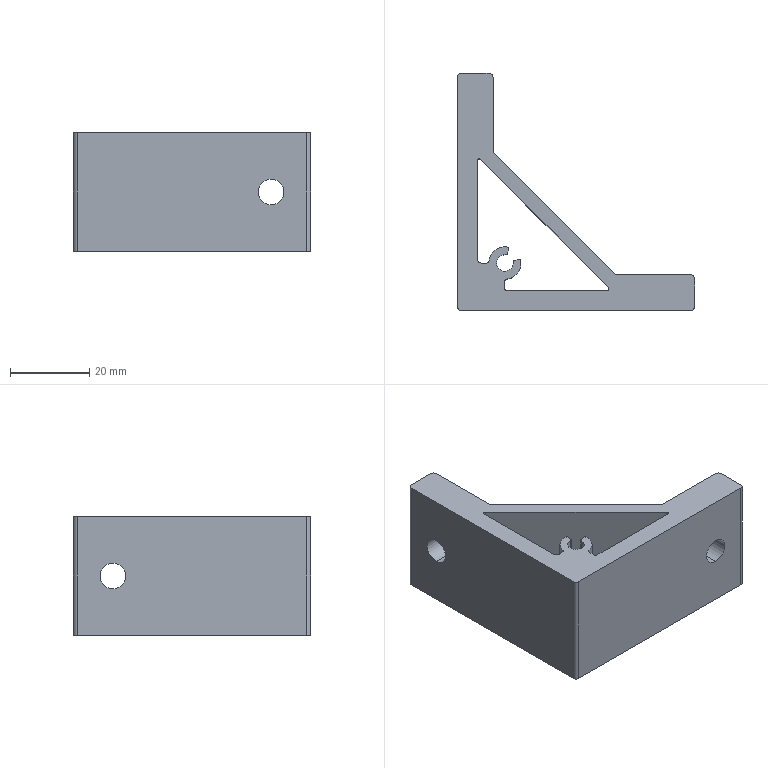Part | SolidWorks | features BaseBody 1 | 1 solid | 41 faces | box 60 x 60 x 30 mm | volume 28435 mm3 | cylinder 25 | plane 16 | commonest cylinder face diameters 1 x10 2 x6 6.5 x4 4.2 x3 8.2 x2
STEP:
#1=CARTESIAN_POINT('',(50.,9.,-11.75));
#2=VERTEX_POINT('',#1);
#3=CARTESIAN_POINT('',(50.,9.,-18.25));
#4=VERTEX_POINT('',#3);
#5=CARTESIAN_POINT('',(50.,9.,-15.));
#6=DIRECTION('',(0.,-1.,0.));
#7=DIRECTION('',(0.,0.,-1.));
#8=AXIS2_PLACEMENT_3D('',#5,#6,#7);
#9=CIRCLE('',#8,3.25);
#10=EDGE_CURVE('',#2,#4,#9,.T.);
#11=ORIENTED_EDGE('',*,*,#10,.F.);
#12=CARTESIAN_POINT('',(50.,0.,-11.75));
#13=VERTEX_POINT('',#12);
#14=CARTESIAN_POINT('',(50.,0.,-11.75));
#15=DIRECTION('',(0.,-1.,0.));
#16=VECTOR('',#15,1000.);
#17=LINE('',#14,#16);
#18=EDGE_CURVE('',#2,#13,#17,.T.);
#19=ORIENTED_EDGE('',*,*,#18,.T.);
#20=CARTESIAN_POINT('',(50.,0.,-18.25));
#21=VERTEX_POINT('',#20);
#22=CARTESIAN_POINT('',(50.,0.,-15.));
#23=DIRECTION('',(0.,1.,0.));
#24=DIRECTION('',(0.,0.,-1.));
#25=AXIS2_PLACEMENT_3D('',#22,#23,#24);
#26=CIRCLE('',#25,3.25);
#27=EDGE_CURVE('',#21,#13,#26,.T.);
#28=ORIENTED_EDGE('',*,*,#27,.F.);
#29=CARTESIAN_POINT('',(50.,0.,-18.25));
#30=DIRECTION('',(0.,-1.,0.));
#31=VECTOR('',#30,1000.);
#32=LINE('',#29,#31);
#33=EDGE_CURVE('',#4,#21,#32,.T.);
#34=ORIENTED_EDGE('',*,*,#33,.F.);
#35=EDGE_LOOP('',(#11,#19,#28,#34));
#36=FACE_OUTER_BOUND('',#35,.T.);
#37=CARTESIAN_POINT('',(50.,0.,-15.));
#38=DIRECTION('',(0.,-1.,0.));
#39=DIRECTION('',(0.,0.,-1.));
#40=AXIS2_PLACEMENT_3D('',#37,#38,#39);
#41=CYLINDRICAL_SURFACE('',#40,3.25);
#42=ADVANCED_FACE('',(#36),#41,.F.);
#43=CARTESIAN_POINT('',(14.101,12.,0.));
#44=VERTEX_POINT('',#43);
#45=CARTESIAN_POINT('',(9.901,12.,0.));
#46=VERTEX_POINT('',#45);
#47=CARTESIAN_POINT('',(12.001,12.,0.));
#48=DIRECTION('',(0.,0.,-1.));
#49=DIRECTION('',(-1.,0.,0.));
#50=AXIS2_PLACEMENT_3D('',#47,#48,#49);
#51=CIRCLE('',#50,2.1);
#52=EDGE_CURVE('',#44,#46,#51,.T.);
#53=ORIENTED_EDGE('',*,*,#52,.F.);
#54=CARTESIAN_POINT('',(14.101,12.,-30.));
#55=VERTEX_POINT('',#54);
#56=CARTESIAN_POINT('',(14.101,12.,-30.));
#57=DIRECTION('',(0.,0.,-1.));
#58=VECTOR('',#57,1000.);
#59=LINE('',#56,#58);
#60=EDGE_CURVE('',#44,#55,#59,.T.);
#61=ORIENTED_EDGE('',*,*,#60,.T.);
#62=CARTESIAN_POINT('',(9.901,12.,-30.));
#63=VERTEX_POINT('',#62);
#64=CARTESIAN_POINT('',(12.001,12.,-30.));
#65=DIRECTION('',(0.,0.,-1.));
#66=DIRECTION('',(-1.,0.,0.));
#67=AXIS2_PLACEMENT_3D('',#64,#65,#66);
#68=CIRCLE('',#67,2.1);
#69=EDGE_CURVE('',#55,#63,#68,.T.);
#70=ORIENTED_EDGE('',*,*,#69,.T.);
#71=CARTESIAN_POINT('',(9.901,12.,-30.));
#72=DIRECTION('',(0.,0.,-1.));
#73=VECTOR('',#72,1000.);
#74=LINE('',#71,#73);
#75=EDGE_CURVE('',#46,#63,#74,.T.);
#76=ORIENTED_EDGE('',*,*,#75,.F.);
#77=EDGE_LOOP('',(#53,#61,#70,#76));
#78=FACE_OUTER_BOUND('',#77,.T.);
#79=CARTESIAN_POINT('',(12.001,12.,-30.));
#80=DIRECTION('',(0.,0.,-1.));
#81=DIRECTION('',(-1.,0.,0.));
#82=AXIS2_PLACEMENT_3D('',#79,#80,#81);
#83=CYLINDRICAL_SURFACE('',#82,2.1);
#84=ADVANCED_FACE('',(#78),#83,.F.);
#85=CARTESIAN_POINT('',(12.144,14.095,0.));
#86=VERTEX_POINT('',#85);
#87=CARTESIAN_POINT('',(12.001,12.,0.));
#88=DIRECTION('',(0.,0.,-1.));
#89=DIRECTION('',(-1.,0.,0.));
#90=AXIS2_PLACEMENT_3D('',#87,#88,#89);
#91=CIRCLE('',#90,2.1);
#92=EDGE_CURVE('',#46,#86,#91,.T.);
#93=ORIENTED_EDGE('',*,*,#92,.F.);
#94=ORIENTED_EDGE('',*,*,#75,.T.);
#95=CARTESIAN_POINT('',(12.144,14.095,-30.));
#96=VERTEX_POINT('',#95);
#97=CARTESIAN_POINT('',(12.001,12.,-30.));
#98=DIRECTION('',(0.,0.,-1.));
#99=DIRECTION('',(-1.,0.,0.));
#100=AXIS2_PLACEMENT_3D('',#97,#98,#99);
#101=CIRCLE('',#100,2.1);
#102=EDGE_CURVE('',#63,#96,#101,.T.);
#103=ORIENTED_EDGE('',*,*,#102,.T.);
#104=CARTESIAN_POINT('',(12.144,14.095,-30.));
#105=DIRECTION('',(0.,0.,-1.));
#106=VECTOR('',#105,1000.);
#107=LINE('',#104,#106);
#108=EDGE_CURVE('',#86,#96,#107,.T.);
#109=ORIENTED_EDGE('',*,*,#108,.F.);
#110=EDGE_LOOP('',(#93,#94,#103,#109));
#111=FACE_OUTER_BOUND('',#110,.T.);
#112=CARTESIAN_POINT('',(12.001,12.,-30.));
#113=DIRECTION('',(0.,0.,-1.));
#114=DIRECTION('',(-1.,0.,0.));
#115=AXIS2_PLACEMENT_3D('',#112,#113,#114);
#116=CYLINDRICAL_SURFACE('',#115,2.1);
#117=ADVANCED_FACE('',(#111),#116,.F.);
#118=CARTESIAN_POINT('',(9.,50.,-11.75));
#119=VERTEX_POINT('',#118);
#120=CARTESIAN_POINT('',(9.,50.,-18.25));
#121=VERTEX_POINT('',#120);
#122=CARTESIAN_POINT('',(9.,50.,-15.));
#123=DIRECTION('',(1.,0.,0.));
#124=DIRECTION('',(0.,0.,1.));
#125=AXIS2_PLACEMENT_3D('',#122,#123,#124);
#126=CIRCLE('',#125,3.25);
#127=EDGE_CURVE('',#119,#121,#126,.T.);
#128=ORIENTED_EDGE('',*,*,#127,.T.);
#129=CARTESIAN_POINT('',(0.,50.,-18.25));
#130=VERTEX_POINT('',#129);
#131=CARTESIAN_POINT('',(0.,50.,-18.25));
#132=DIRECTION('',(-1.,0.,0.));
#133=VECTOR('',#132,1000.);
#134=LINE('',#131,#133);
#135=EDGE_CURVE('',#121,#130,#134,.T.);
#136=ORIENTED_EDGE('',*,*,#135,.T.);
#137=CARTESIAN_POINT('',(0.,50.,-11.75));
#138=VERTEX_POINT('',#137);
#139=CARTESIAN_POINT('',(0.,50.,-15.));
#140=DIRECTION('',(1.,0.,0.));
#141=DIRECTION('',(0.,0.,1.));
#142=AXIS2_PLACEMENT_3D('',#139,#140,#141);
#143=CIRCLE('',#142,3.25);
#144=EDGE_CURVE('',#138,#130,#143,.T.);
#145=ORIENTED_EDGE('',*,*,#144,.F.);
#146=CARTESIAN_POINT('',(0.,50.,-11.75));
#147=DIRECTION('',(-1.,0.,0.));
#148=VECTOR('',#147,1000.);
#149=LINE('',#146,#148);
#150=EDGE_CURVE('',#119,#138,#149,.T.);
#151=ORIENTED_EDGE('',*,*,#150,.F.);
#152=EDGE_LOOP('',(#128,#136,#145,#151));
#153=FACE_OUTER_BOUND('',#152,.T.);
#154=CARTESIAN_POINT('',(0.,50.,-15.));
#155=DIRECTION('',(-1.,0.,0.));
#156=DIRECTION('',(0.,0.,1.));
#157=AXIS2_PLACEMENT_3D('',#154,#155,#156);
#158=CYLINDRICAL_SURFACE('',#157,3.25);
#159=ADVANCED_FACE('',(#153),#158,.F.);
#160=CARTESIAN_POINT('',(14.096,12.143,0.));
#161=VERTEX_POINT('',#160);
#162=CARTESIAN_POINT('',(14.095,12.177,0.));
#163=VERTEX_POINT('',#162);
#164=CARTESIAN_POINT('',(14.595,12.177,0.));
#165=DIRECTION('',(0.,0.,-1.));
#166=DIRECTION('',(-1.,0.,0.));
#167=AXIS2_PLACEMENT_3D('',#164,#165,#166);
#168=CIRCLE('',#167,0.5);
#169=EDGE_CURVE('',#161,#163,#168,.T.);
#170=ORIENTED_EDGE('',*,*,#169,.T.);
#171=CARTESIAN_POINT('',(14.095,12.177,-30.));
#172=VERTEX_POINT('',#171);
#173=CARTESIAN_POINT('',(14.095,12.177,-30.));
#174=DIRECTION('',(0.,0.,-1.));
#175=VECTOR('',#174,1000.);
#176=LINE('',#173,#175);
#177=EDGE_CURVE('',#163,#172,#176,.T.);
#178=ORIENTED_EDGE('',*,*,#177,.T.);
#179=CARTESIAN_POINT('',(14.096,12.143,-30.));
#180=VERTEX_POINT('',#179);
#181=CARTESIAN_POINT('',(14.595,12.177,-30.));
#182=DIRECTION('',(0.,0.,1.));
#183=DIRECTION('',(-1.,0.,0.));
#184=AXIS2_PLACEMENT_3D('',#181,#182,#183);
#185=CIRCLE('',#184,0.5);
#186=EDGE_CURVE('',#172,#180,#185,.T.);
#187=ORIENTED_EDGE('',*,*,#186,.T.);
#188=CARTESIAN_POINT('',(14.096,12.143,-30.));
#189=DIRECTION('',(0.,0.,1.));
#190=VECTOR('',#189,1000.);
#191=LINE('',#188,#190);
#192=EDGE_CURVE('',#180,#161,#191,.T.);
#193=ORIENTED_EDGE('',*,*,#192,.T.);
#194=EDGE_LOOP('',(#170,#178,#187,#193));
#195=FACE_OUTER_BOUND('',#194,.T.);
#196=CARTESIAN_POINT('',(14.595,12.177,-30.));
#197=DIRECTION('',(0.,0.,-1.));
#198=DIRECTION('',(-1.,0.,0.));
#199=AXIS2_PLACEMENT_3D('',#196,#197,#198);
#200=CYLINDRICAL_SURFACE('',#199,0.5);
#201=ADVANCED_FACE('',(#195),#200,.T.);
#202=CARTESIAN_POINT('',(59.,0.,0.));
#203=VERTEX_POINT('',#202);
#204=CARTESIAN_POINT('',(1.,0.,0.));
#205=VERTEX_POINT('',#204);
#206=CARTESIAN_POINT('',(0.,0.,0.));
#207=DIRECTION('',(-1.,0.,0.));
#208=VECTOR('',#207,1000.);
#209=LINE('',#206,#208);
#210=EDGE_CURVE('',#203,#205,#209,.T.);
#211=ORIENTED_EDGE('',*,*,#210,.T.);
#212=CARTESIAN_POINT('',(1.,0.,-30.));
#213=VERTEX_POINT('',#212);
#214=CARTESIAN_POINT('',(1.,0.,-30.));
#215=DIRECTION('',(0.,0.,-1.));
#216=VECTOR('',#215,1000.);
#217=LINE('',#214,#216);
#218=EDGE_CURVE('',#205,#213,#217,.T.);
#219=ORIENTED_EDGE('',*,*,#218,.T.);
#220=CARTESIAN_POINT('',(59.,0.,-30.));
#221=VERTEX_POINT('',#220);
#222=CARTESIAN_POINT('',(0.,0.,-30.));
#223=DIRECTION('',(1.,0.,0.));
#224=VECTOR('',#223,1000.);
#225=LINE('',#222,#224);
#226=EDGE_CURVE('',#213,#221,#225,.T.);
#227=ORIENTED_EDGE('',*,*,#226,.T.);
#228=CARTESIAN_POINT('',(59.,0.,-30.));
#229=DIRECTION('',(0.,0.,1.));
#230=VECTOR('',#229,1000.);
#231=LINE('',#228,#230);
#232=EDGE_CURVE('',#221,#203,#231,.T.);
#233=ORIENTED_EDGE('',*,*,#232,.T.);
#234=EDGE_LOOP('',(#211,#219,#227,#233));
#235=FACE_OUTER_BOUND('',#234,.T.);
#236=ORIENTED_EDGE('',*,*,#27,.T.);
#237=CARTESIAN_POINT('',(50.,0.,-15.));
#238=DIRECTION('',(0.,1.,0.));
#239=DIRECTION('',(0.,0.,-1.));
#240=AXIS2_PLACEMENT_3D('',#237,#238,#239);
#241=CIRCLE('',#240,3.25);
#242=EDGE_CURVE('',#13,#21,#241,.T.);
#243=ORIENTED_EDGE('',*,*,#242,.T.);
#244=EDGE_LOOP('',(#236,#243));
#245=FACE_BOUND('',#244,.T.);
#246=CARTESIAN_POINT('',(0.,0.,-30.));
#247=DIRECTION('',(0.,-1.,0.));
#248=DIRECTION('',(0.,0.,-1.));
#249=AXIS2_PLACEMENT_3D('',#246,#247,#248);
#250=PLANE('',#249);
#251=ADVANCED_FACE('',(#235,#245),#250,.T.);
#252=CARTESIAN_POINT('',(0.,1.,0.));
#253=VERTEX_POINT('',#252);
#254=CARTESIAN_POINT('',(1.,1.,0.));
#255=DIRECTION('',(0.,0.,-1.));
#256=DIRECTION('',(1.,0.,0.));
#257=AXIS2_PLACEMENT_3D('',#254,#255,#256);
#258=CIRCLE('',#257,1.);
#259=EDGE_CURVE('',#205,#253,#258,.T.);
#260=ORIENTED_EDGE('',*,*,#259,.T.);
#261=CARTESIAN_POINT('',(0.,1.,-30.));
#262=VERTEX_POINT('',#261);
#263=CARTESIAN_POINT('',(0.,1.,-30.));
#264=DIRECTION('',(0.,0.,-1.));
#265=VECTOR('',#264,1000.);
#266=LINE('',#263,#265);
#267=EDGE_CURVE('',#253,#262,#266,.T.);
#268=ORIENTED_EDGE('',*,*,#267,.T.);
#269=CARTESIAN_POINT('',(1.,1.,-30.));
#270=DIRECTION('',(0.,0.,1.));
#271=DIRECTION('',(1.,0.,0.));
#272=AXIS2_PLACEMENT_3D('',#269,#270,#271);
#273=CIRCLE('',#272,1.);
#274=EDGE_CURVE('',#262,#213,#273,.T.);
#275=ORIENTED_EDGE('',*,*,#274,.T.);
#276=ORIENTED_EDGE('',*,*,#218,.F.);
#277=EDGE_LOOP('',(#260,#268,#275,#276));
#278=FACE_OUTER_BOUND('',#277,.T.);
#279=CARTESIAN_POINT('',(1.,1.,-30.));
#280=DIRECTION('',(0.,0.,1.));
#281=DIRECTION('',(1.,0.,0.));
#282=AXIS2_PLACEMENT_3D('',#279,#280,#281);
#283=CYLINDRICAL_SURFACE('',#282,1.);
#284=ADVANCED_FACE('',(#278),#283,.T.);
#285=ORIENTED_EDGE('',*,*,#210,.F.);
#286=CARTESIAN_POINT('',(60.,1.,0.));
#287=VERTEX_POINT('',#286);
#288=CARTESIAN_POINT('',(59.,1.,0.));
#289=DIRECTION('',(0.,0.,1.));
#290=DIRECTION('',(1.,0.,0.));
#291=AXIS2_PLACEMENT_3D('',#288,#289,#290);
#292=CIRCLE('',#291,1.);
#293=EDGE_CURVE('',#203,#287,#292,.T.);
#294=ORIENTED_EDGE('',*,*,#293,.T.);
#295=CARTESIAN_POINT('',(60.,8.,0.));
#296=VERTEX_POINT('',#295);
#297=CARTESIAN_POINT('',(60.,0.,0.));
#298=DIRECTION('',(0.,1.,0.));
#299=VECTOR('',#298,1000.);
#300=LINE('',#297,#299);
#301=EDGE_CURVE('',#287,#296,#300,.T.);
#302=ORIENTED_EDGE('',*,*,#301,.T.);
#303=CARTESIAN_POINT('',(59.,9.,0.));
#304=VERTEX_POINT('',#303);
#305=CARTESIAN_POINT('',(59.,8.,0.));
#306=DIRECTION('',(0.,0.,-1.));
#307=DIRECTION('',(1.,0.,0.));
#308=AXIS2_PLACEMENT_3D('',#305,#306,#307);
#309=CIRCLE('',#308,1.);
#310=EDGE_CURVE('',#304,#296,#309,.T.);
#311=ORIENTED_EDGE('',*,*,#310,.F.);
#312=CARTESIAN_POINT('',(40.,9.,0.));
#313=VERTEX_POINT('',#312);
#314=CARTESIAN_POINT('',(0.,9.,0.));
#315=DIRECTION('',(-1.,0.,0.));
#316=VECTOR('',#315,1000.);
#317=LINE('',#314,#316);
#318=EDGE_CURVE('',#304,#313,#317,.T.);
#319=ORIENTED_EDGE('',*,*,#318,.T.);
#320=CARTESIAN_POINT('',(9.,40.,0.));
#321=VERTEX_POINT('',#320);
#322=CARTESIAN_POINT('',(40.,9.,0.));
#323=DIRECTION('',(-0.7071,0.7071,0.));
#324=VECTOR('',#323,1000.);
#325=LINE('',#322,#324);
#326=EDGE_CURVE('',#313,#321,#325,.T.);
#327=ORIENTED_EDGE('',*,*,#326,.T.);
#328=CARTESIAN_POINT('',(9.,59.,0.));
#329=VERTEX_POINT('',#328);
#330=CARTESIAN_POINT('',(9.,0.,0.));
#331=DIRECTION('',(0.,1.,0.));
#332=VECTOR('',#331,1000.);
#333=LINE('',#330,#332);
#334=EDGE_CURVE('',#321,#329,#333,.T.);
#335=ORIENTED_EDGE('',*,*,#334,.T.);
#336=CARTESIAN_POINT('',(8.,60.,0.));
#337=VERTEX_POINT('',#336);
#338=CARTESIAN_POINT('',(8.,59.,0.));
#339=DIRECTION('',(0.,0.,-1.));
#340=DIRECTION('',(1.,0.,0.));
#341=AXIS2_PLACEMENT_3D('',#338,#339,#340);
#342=CIRCLE('',#341,1.);
#343=EDGE_CURVE('',#337,#329,#342,.T.);
#344=ORIENTED_EDGE('',*,*,#343,.F.);
#345=CARTESIAN_POINT('',(1.,60.,0.));
#346=VERTEX_POINT('',#345);
#347=CARTESIAN_POINT('',(0.,60.,0.));
#348=DIRECTION('',(-1.,0.,0.));
#349=VECTOR('',#348,1000.);
#350=LINE('',#347,#349);
#351=EDGE_CURVE('',#337,#346,#350,.T.);
#352=ORIENTED_EDGE('',*,*,#351,.T.);
#353=CARTESIAN_POINT('',(0.,59.,0.));
#354=VERTEX_POINT('',#353);
#355=CARTESIAN_POINT('',(1.,59.,0.));
#356=DIRECTION('',(0.,0.,-1.));
#357=DIRECTION('',(1.,0.,0.));
#358=AXIS2_PLACEMENT_3D('',#355,#356,#357);
#359=CIRCLE('',#358,1.);
#360=EDGE_CURVE('',#354,#346,#359,.T.);
#361=ORIENTED_EDGE('',*,*,#360,.F.);
#362=CARTESIAN_POINT('',(0.,0.,0.));
#363=DIRECTION('',(0.,-1.,0.));
#364=VECTOR('',#363,1000.);
#365=LINE('',#362,#364);
#366=EDGE_CURVE('',#354,#253,#365,.T.);
#367=ORIENTED_EDGE('',*,*,#366,.T.);
#368=ORIENTED_EDGE('',*,*,#259,.F.);
#369=EDGE_LOOP('',(#285,#294,#302,#311,#319,#327,#335,#344,#352,#361,#367,#368));
#370=FACE_OUTER_BOUND('',#369,.T.);
#371=CARTESIAN_POINT('',(12.446,7.924,0.));
#372=VERTEX_POINT('',#371);
#373=CARTESIAN_POINT('',(16.07,12.5,0.));
#374=VERTEX_POINT('',#373);
#375=CARTESIAN_POINT('',(12.001,12.,0.));
#376=DIRECTION('',(0.,0.,1.));
#377=DIRECTION('',(-1.,0.,0.));
#378=AXIS2_PLACEMENT_3D('',#375,#376,#377);
#379=CIRCLE('',#378,4.1);
#380=EDGE_CURVE('',#372,#374,#379,.T.);
#381=ORIENTED_EDGE('',*,*,#380,.T.);
#382=CARTESIAN_POINT('',(15.445,12.922,0.));
#383=VERTEX_POINT('',#382);
#384=CARTESIAN_POINT('',(15.574,12.439,0.));
#385=DIRECTION('',(0.,0.,-1.));
#386=DIRECTION('',(-1.,0.,0.));
#387=AXIS2_PLACEMENT_3D('',#384,#385,#386);
#388=CIRCLE('',#387,0.5);
#389=EDGE_CURVE('',#383,#374,#388,.T.);
#390=ORIENTED_EDGE('',*,*,#389,.F.);
#391=CARTESIAN_POINT('',(14.466,12.66,0.));
#392=VERTEX_POINT('',#391);
#393=CARTESIAN_POINT('',(15.961,13.06,0.));
#394=DIRECTION('',(-0.966,-0.2585,0.));
#395=VECTOR('',#394,1000.);
#396=LINE('',#393,#395);
#397=EDGE_CURVE('',#383,#392,#396,.T.);
#398=ORIENTED_EDGE('',*,*,#397,.T.);
#399=CARTESIAN_POINT('',(14.595,12.177,0.));
#400=DIRECTION('',(0.,0.,-1.));
#401=DIRECTION('',(-1.,0.,0.));
#402=AXIS2_PLACEMENT_3D('',#399,#400,#401);
#403=CIRCLE('',#402,0.5);
#404=EDGE_CURVE('',#163,#392,#403,.T.);
#405=ORIENTED_EDGE('',*,*,#404,.F.);
#406=ORIENTED_EDGE('',*,*,#169,.F.);
#407=CARTESIAN_POINT('',(12.001,12.,0.));
#408=DIRECTION('',(0.,0.,-1.));
#409=DIRECTION('',(-1.,0.,0.));
#410=AXIS2_PLACEMENT_3D('',#407,#408,#409);
#411=CIRCLE('',#410,2.1);
#412=EDGE_CURVE('',#161,#44,#411,.T.);
#413=ORIENTED_EDGE('',*,*,#412,.T.);
#414=ORIENTED_EDGE('',*,*,#52,.T.);
#415=ORIENTED_EDGE('',*,*,#92,.T.);
#416=CARTESIAN_POINT('',(12.661,14.465,0.));
#417=VERTEX_POINT('',#416);
#418=CARTESIAN_POINT('',(12.178,14.594,0.));
#419=DIRECTION('',(0.,0.,-1.));
#420=DIRECTION('',(-1.,0.,0.));
#421=AXIS2_PLACEMENT_3D('',#418,#419,#420);
#422=CIRCLE('',#421,0.5);
#423=EDGE_CURVE('',#417,#86,#422,.T.);
#424=ORIENTED_EDGE('',*,*,#423,.F.);
#425=CARTESIAN_POINT('',(12.923,15.443,0.));
#426=VERTEX_POINT('',#425);
#427=CARTESIAN_POINT('',(12.002,12.001,0.));
#428=DIRECTION('',(0.2585,0.966,0.));
#429=VECTOR('',#428,1000.);
#430=LINE('',#427,#429);
#431=EDGE_CURVE('',#417,#426,#430,.T.);
#432=ORIENTED_EDGE('',*,*,#431,.T.);
#433=CARTESIAN_POINT('',(12.501,16.069,0.));
#434=VERTEX_POINT('',#433);
#435=CARTESIAN_POINT('',(12.44,15.573,0.));
#436=DIRECTION('',(0.,0.,-1.));
#437=DIRECTION('',(-1.,0.,0.));
#438=AXIS2_PLACEMENT_3D('',#435,#436,#437);
#439=CIRCLE('',#438,0.5);
#440=EDGE_CURVE('',#434,#426,#439,.T.);
#441=ORIENTED_EDGE('',*,*,#440,.F.);
#442=CARTESIAN_POINT('',(7.925,12.445,0.));
#443=VERTEX_POINT('',#442);
#444=CARTESIAN_POINT('',(12.001,12.,0.));
#445=DIRECTION('',(0.,0.,1.));
#446=DIRECTION('',(-1.,0.,0.));
#447=AXIS2_PLACEMENT_3D('',#444,#445,#446);
#448=CIRCLE('',#447,4.1);
#449=EDGE_CURVE('',#434,#443,#448,.T.);
#450=ORIENTED_EDGE('',*,*,#449,.T.);
#451=CARTESIAN_POINT('',(7.428,12.,0.));
#452=VERTEX_POINT('',#451);
#453=CARTESIAN_POINT('',(7.428,12.5,0.));
#454=DIRECTION('',(0.,0.,-1.));
#455=DIRECTION('',(-1.,0.,0.));
#456=AXIS2_PLACEMENT_3D('',#453,#454,#455);
#457=CIRCLE('',#456,0.5);
#458=EDGE_CURVE('',#443,#452,#457,.T.);
#459=ORIENTED_EDGE('',*,*,#458,.T.);
#460=CARTESIAN_POINT('',(6.,12.,0.));
#461=VERTEX_POINT('',#460);
#462=CARTESIAN_POINT('',(7.901,12.,0.));
#463=DIRECTION('',(-1.,0.,0.));
#464=VECTOR('',#463,1000.);
#465=LINE('',#462,#464);
#466=EDGE_CURVE('',#452,#461,#465,.T.);
#467=ORIENTED_EDGE('',*,*,#466,.T.);
#468=CARTESIAN_POINT('',(5.,13.,0.));
#469=VERTEX_POINT('',#468);
#470=CARTESIAN_POINT('',(6.,13.,0.));
#471=DIRECTION('',(0.,0.,-1.));
#472=DIRECTION('',(1.,0.,0.));
#473=AXIS2_PLACEMENT_3D('',#470,#471,#472);
#474=CIRCLE('',#473,1.);
#475=EDGE_CURVE('',#461,#469,#474,.T.);
#476=ORIENTED_EDGE('',*,*,#475,.T.);
#477=CARTESIAN_POINT('',(5.,37.843,0.));
#478=VERTEX_POINT('',#477);
#479=CARTESIAN_POINT('',(5.,0.,0.));
#480=DIRECTION('',(0.,1.,0.));
#481=VECTOR('',#480,1000.);
#482=LINE('',#479,#481);
#483=EDGE_CURVE('',#469,#478,#482,.T.);
#484=ORIENTED_EDGE('',*,*,#483,.T.);
#485=CARTESIAN_POINT('',(5.854,38.196,0.));
#486=VERTEX_POINT('',#485);
#487=CARTESIAN_POINT('',(5.5,37.843,0.));
#488=DIRECTION('',(0.,0.,-1.));
#489=DIRECTION('',(-1.,0.,0.));
#490=AXIS2_PLACEMENT_3D('',#487,#488,#489);
#491=CIRCLE('',#490,0.5);
#492=EDGE_CURVE('',#478,#486,#491,.T.);
#493=ORIENTED_EDGE('',*,*,#492,.T.);
#494=CARTESIAN_POINT('',(38.196,5.854,0.));
#495=VERTEX_POINT('',#494);
#496=CARTESIAN_POINT('',(5.854,38.196,0.));
#497=DIRECTION('',(0.7071,-0.7071,0.));
#498=VECTOR('',#497,1000.);
#499=LINE('',#496,#498);
#500=EDGE_CURVE('',#486,#495,#499,.T.);
#501=ORIENTED_EDGE('',*,*,#500,.T.);
#502=CARTESIAN_POINT('',(37.844,5.,0.));
#503=VERTEX_POINT('',#502);
#504=CARTESIAN_POINT('',(37.843,5.5,0.));
#505=DIRECTION('',(0.,0.,-1.));
#506=DIRECTION('',(-1.,0.,0.));
#507=AXIS2_PLACEMENT_3D('',#504,#505,#506);
#508=CIRCLE('',#507,0.5);
#509=EDGE_CURVE('',#495,#503,#508,.T.);
#510=ORIENTED_EDGE('',*,*,#509,.T.);
#511=CARTESIAN_POINT('',(12.5,5.,0.));
#512=VERTEX_POINT('',#511);
#513=CARTESIAN_POINT('',(0.,5.,0.));
#514=DIRECTION('',(-1.,0.,0.));
#515=VECTOR('',#514,1000.);
#516=LINE('',#513,#515);
#517=EDGE_CURVE('',#503,#512,#516,.T.);
#518=ORIENTED_EDGE('',*,*,#517,.T.);
#519=CARTESIAN_POINT('',(12.,5.5,0.));
#520=VERTEX_POINT('',#519);
#521=CARTESIAN_POINT('',(12.5,5.5,0.));
#522=DIRECTION('',(0.,0.,-1.));
#523=DIRECTION('',(1.,0.,0.));
#524=AXIS2_PLACEMENT_3D('',#521,#522,#523);
#525=CIRCLE('',#524,0.5);
#526=EDGE_CURVE('',#512,#520,#525,.T.);
#527=ORIENTED_EDGE('',*,*,#526,.T.);
#528=CARTESIAN_POINT('',(12.,7.427,0.));
#529=VERTEX_POINT('',#528);
#530=CARTESIAN_POINT('',(12.,0.,0.));
#531=DIRECTION('',(0.,1.,0.));
#532=VECTOR('',#531,1000.);
#533=LINE('',#530,#532);
#534=EDGE_CURVE('',#520,#529,#533,.T.);
#535=ORIENTED_EDGE('',*,*,#534,.T.);
#536=CARTESIAN_POINT('',(12.5,7.427,0.));
#537=DIRECTION('',(0.,0.,-1.));
#538=DIRECTION('',(-1.,0.,0.));
#539=AXIS2_PLACEMENT_3D('',#536,#537,#538);
#540=CIRCLE('',#539,0.5);
#541=EDGE_CURVE('',#529,#372,#540,.T.);
#542=ORIENTED_EDGE('',*,*,#541,.T.);
#543=EDGE_LOOP('',(#381,#390,#398,#405,#406,#413,#414,#415,#424,#432,#441,#450,#459,#467,#476,#484,#493,#501,#510,#518,#527,#535,#542));
#544=FACE_BOUND('',#543,.T.);
#545=CARTESIAN_POINT('',(0.,0.,0.));
#546=DIRECTION('',(0.,0.,1.));
#547=DIRECTION('',(1.,0.,0.));
#548=AXIS2_PLACEMENT_3D('',#545,#546,#547);
#549=PLANE('',#548);
#550=ADVANCED_FACE('',(#370,#544),#549,.T.);
#551=ORIENTED_EDGE('',*,*,#293,.F.);
#552=ORIENTED_EDGE('',*,*,#232,.F.);
#553=CARTESIAN_POINT('',(60.,1.,-30.));
#554=VERTEX_POINT('',#553);
#555=CARTESIAN_POINT('',(59.,1.,-30.));
#556=DIRECTION('',(0.,0.,1.));
#557=DIRECTION('',(1.,0.,0.));
#558=AXIS2_PLACEMENT_3D('',#555,#556,#557);
#559=CIRCLE('',#558,1.);
#560=EDGE_CURVE('',#221,#554,#559,.T.);
#561=ORIENTED_EDGE('',*,*,#560,.T.);
#562=CARTESIAN_POINT('',(60.,1.,-30.));
#563=DIRECTION('',(0.,0.,1.));
#564=VECTOR('',#563,1000.);
#565=LINE('',#562,#564);
#566=EDGE_CURVE('',#554,#287,#565,.T.);
#567=ORIENTED_EDGE('',*,*,#566,.T.);
#568=EDGE_LOOP('',(#551,#552,#561,#567));
#569=FACE_OUTER_BOUND('',#568,.T.);
#570=CARTESIAN_POINT('',(59.,1.,-30.));
#571=DIRECTION('',(0.,0.,1.));
#572=DIRECTION('',(1.,0.,0.));
#573=AXIS2_PLACEMENT_3D('',#570,#571,#572);
#574=CYLINDRICAL_SURFACE('',#573,1.);
#575=ADVANCED_FACE('',(#569),#574,.T.);
#576=CARTESIAN_POINT('',(60.,8.,-30.));
#577=VERTEX_POINT('',#576);
#578=CARTESIAN_POINT('',(59.,9.,-30.));
#579=VERTEX_POINT('',#578);
#580=CARTESIAN_POINT('',(59.,8.,-30.));
#581=DIRECTION('',(0.,0.,1.));
#582=DIRECTION('',(1.,0.,0.));
#583=AXIS2_PLACEMENT_3D('',#580,#581,#582);
#584=CIRCLE('',#583,1.);
#585=EDGE_CURVE('',#577,#579,#584,.T.);
#586=ORIENTED_EDGE('',*,*,#585,.F.);
#587=CARTESIAN_POINT('',(60.,0.,-30.));
#588=DIRECTION('',(0.,1.,0.));
#589=VECTOR('',#588,1000.);
#590=LINE('',#587,#589);
#591=EDGE_CURVE('',#554,#577,#590,.T.);
#592=ORIENTED_EDGE('',*,*,#591,.F.);
#593=ORIENTED_EDGE('',*,*,#560,.F.);
#594=ORIENTED_EDGE('',*,*,#226,.F.);
#595=ORIENTED_EDGE('',*,*,#274,.F.);
#596=CARTESIAN_POINT('',(0.,59.,-30.));
#597=VERTEX_POINT('',#596);
#598=CARTESIAN_POINT('',(0.,0.,-30.));
#599=DIRECTION('',(0.,-1.,0.));
#600=VECTOR('',#599,1000.);
#601=LINE('',#598,#600);
#602=EDGE_CURVE('',#597,#262,#601,.T.);
#603=ORIENTED_EDGE('',*,*,#602,.F.);
#604=CARTESIAN_POINT('',(1.,60.,-30.));
#605=VERTEX_POINT('',#604);
#606=CARTESIAN_POINT('',(1.,59.,-30.));
#607=DIRECTION('',(0.,0.,1.));
#608=DIRECTION('',(1.,0.,0.));
#609=AXIS2_PLACEMENT_3D('',#606,#607,#608);
#610=CIRCLE('',#609,1.);
#611=EDGE_CURVE('',#605,#597,#610,.T.);
#612=ORIENTED_EDGE('',*,*,#611,.F.);
#613=CARTESIAN_POINT('',(8.,60.,-30.));
#614=VERTEX_POINT('',#613);
#615=CARTESIAN_POINT('',(0.,60.,-30.));
#616=DIRECTION('',(-1.,0.,0.));
#617=VECTOR('',#616,1000.);
#618=LINE('',#615,#617);
#619=EDGE_CURVE('',#614,#605,#618,.T.);
#620=ORIENTED_EDGE('',*,*,#619,.F.);
#621=CARTESIAN_POINT('',(9.,59.,-30.));
#622=VERTEX_POINT('',#621);
#623=CARTESIAN_POINT('',(8.,59.,-30.));
#624=DIRECTION('',(0.,0.,1.));
#625=DIRECTION('',(1.,0.,0.));
#626=AXIS2_PLACEMENT_3D('',#623,#624,#625);
#627=CIRCLE('',#626,1.);
#628=EDGE_CURVE('',#622,#614,#627,.T.);
#629=ORIENTED_EDGE('',*,*,#628,.F.);
#630=CARTESIAN_POINT('',(9.,40.,-30.));
#631=VERTEX_POINT('',#630);
#632=CARTESIAN_POINT('',(9.,0.,-30.));
#633=DIRECTION('',(0.,1.,0.));
#634=VECTOR('',#633,1000.);
#635=LINE('',#632,#634);
#636=EDGE_CURVE('',#631,#622,#635,.T.);
#637=ORIENTED_EDGE('',*,*,#636,.F.);
#638=CARTESIAN_POINT('',(40.,9.,-30.));
#639=VERTEX_POINT('',#638);
#640=CARTESIAN_POINT('',(40.,9.,-30.));
#641=DIRECTION('',(-0.7071,0.7071,0.));
#642=VECTOR('',#641,1000.);
#643=LINE('',#640,#642);
#644=EDGE_CURVE('',#639,#631,#643,.T.);
#645=ORIENTED_EDGE('',*,*,#644,.F.);
#646=CARTESIAN_POINT('',(0.,9.,-30.));
#647=DIRECTION('',(-1.,0.,0.));
#648=VECTOR('',#647,1000.);
#649=LINE('',#646,#648);
#650=EDGE_CURVE('',#579,#639,#649,.T.);
#651=ORIENTED_EDGE('',*,*,#650,.F.);
#652=EDGE_LOOP('',(#586,#592,#593,#594,#595,#603,#612,#620,#629,#637,#645,#651));
#653=FACE_OUTER_BOUND('',#652,.T.);
#654=CARTESIAN_POINT('',(14.466,12.66,-30.));
#655=VERTEX_POINT('',#654);
#656=CARTESIAN_POINT('',(14.595,12.177,-30.));
#657=DIRECTION('',(0.,0.,1.));
#658=DIRECTION('',(-1.,0.,0.));
#659=AXIS2_PLACEMENT_3D('',#656,#657,#658);
#660=CIRCLE('',#659,0.5);
#661=EDGE_CURVE('',#655,#172,#660,.T.);
#662=ORIENTED_EDGE('',*,*,#661,.F.);
#663=CARTESIAN_POINT('',(15.445,12.922,-30.));
#664=VERTEX_POINT('',#663);
#665=CARTESIAN_POINT('',(15.961,13.06,-30.));
#666=DIRECTION('',(0.966,0.2585,0.));
#667=VECTOR('',#666,1000.);
#668=LINE('',#665,#667);
#669=EDGE_CURVE('',#655,#664,#668,.T.);
#670=ORIENTED_EDGE('',*,*,#669,.T.);
#671=CARTESIAN_POINT('',(16.07,12.5,-30.));
#672=VERTEX_POINT('',#671);
#673=CARTESIAN_POINT('',(15.574,12.439,-30.));
#674=DIRECTION('',(0.,0.,1.));
#675=DIRECTION('',(-1.,0.,0.));
#676=AXIS2_PLACEMENT_3D('',#673,#674,#675);
#677=CIRCLE('',#676,0.5);
#678=EDGE_CURVE('',#672,#664,#677,.T.);
#679=ORIENTED_EDGE('',*,*,#678,.F.);
#680=CARTESIAN_POINT('',(12.446,7.924,-30.));
#681=VERTEX_POINT('',#680);
#682=CARTESIAN_POINT('',(12.001,12.,-30.));
#683=DIRECTION('',(0.,0.,1.));
#684=DIRECTION('',(-1.,0.,0.));
#685=AXIS2_PLACEMENT_3D('',#682,#683,#684);
#686=CIRCLE('',#685,4.1);
#687=EDGE_CURVE('',#681,#672,#686,.T.);
#688=ORIENTED_EDGE('',*,*,#687,.F.);
#689=CARTESIAN_POINT('',(12.,7.427,-30.));
#690=VERTEX_POINT('',#689);
#691=CARTESIAN_POINT('',(12.5,7.427,-30.));
#692=DIRECTION('',(0.,0.,1.));
#693=DIRECTION('',(-1.,0.,0.));
#694=AXIS2_PLACEMENT_3D('',#691,#692,#693);
#695=CIRCLE('',#694,0.5);
#696=EDGE_CURVE('',#681,#690,#695,.T.);
#697=ORIENTED_EDGE('',*,*,#696,.T.);
#698=CARTESIAN_POINT('',(12.,5.5,-30.));
#699=VERTEX_POINT('',#698);
#700=CARTESIAN_POINT('',(12.,0.,-30.));
#701=DIRECTION('',(0.,1.,0.));
#702=VECTOR('',#701,1000.);
#703=LINE('',#700,#702);
#704=EDGE_CURVE('',#699,#690,#703,.T.);
#705=ORIENTED_EDGE('',*,*,#704,.F.);
#706=CARTESIAN_POINT('',(12.5,5.,-30.));
#707=VERTEX_POINT('',#706);
#708=CARTESIAN_POINT('',(12.5,5.5,-30.));
#709=DIRECTION('',(0.,0.,1.));
#710=DIRECTION('',(1.,0.,0.));
#711=AXIS2_PLACEMENT_3D('',#708,#709,#710);
#712=CIRCLE('',#711,0.5);
#713=EDGE_CURVE('',#699,#707,#712,.T.);
#714=ORIENTED_EDGE('',*,*,#713,.T.);
#715=CARTESIAN_POINT('',(37.844,5.,-30.));
#716=VERTEX_POINT('',#715);
#717=CARTESIAN_POINT('',(0.,5.,-30.));
#718=DIRECTION('',(-1.,0.,0.));
#719=VECTOR('',#718,1000.);
#720=LINE('',#717,#719);
#721=EDGE_CURVE('',#716,#707,#720,.T.);
#722=ORIENTED_EDGE('',*,*,#721,.F.);
#723=CARTESIAN_POINT('',(38.196,5.854,-30.));
#724=VERTEX_POINT('',#723);
#725=CARTESIAN_POINT('',(37.843,5.5,-30.));
#726=DIRECTION('',(0.,0.,1.));
#727=DIRECTION('',(-1.,0.,0.));
#728=AXIS2_PLACEMENT_3D('',#725,#726,#727);
#729=CIRCLE('',#728,0.5);
#730=EDGE_CURVE('',#716,#724,#729,.T.);
#731=ORIENTED_EDGE('',*,*,#730,.T.);
#732=CARTESIAN_POINT('',(5.854,38.196,-30.));
#733=VERTEX_POINT('',#732);
#734=CARTESIAN_POINT('',(5.854,38.196,-30.));
#735=DIRECTION('',(0.7071,-0.7071,0.));
#736=VECTOR('',#735,1000.);
#737=LINE('',#734,#736);
#738=EDGE_CURVE('',#733,#724,#737,.T.);
#739=ORIENTED_EDGE('',*,*,#738,.F.);
#740=CARTESIAN_POINT('',(5.,37.843,-30.));
#741=VERTEX_POINT('',#740);
#742=CARTESIAN_POINT('',(5.5,37.843,-30.));
#743=DIRECTION('',(0.,0.,1.));
#744=DIRECTION('',(-1.,0.,0.));
#745=AXIS2_PLACEMENT_3D('',#742,#743,#744);
#746=CIRCLE('',#745,0.5);
#747=EDGE_CURVE('',#733,#741,#746,.T.);
#748=ORIENTED_EDGE('',*,*,#747,.T.);
#749=CARTESIAN_POINT('',(5.,13.,-30.));
#750=VERTEX_POINT('',#749);
#751=CARTESIAN_POINT('',(5.,0.,-30.));
#752=DIRECTION('',(0.,1.,0.));
#753=VECTOR('',#752,1000.);
#754=LINE('',#751,#753);
#755=EDGE_CURVE('',#750,#741,#754,.T.);
#756=ORIENTED_EDGE('',*,*,#755,.F.);
#757=CARTESIAN_POINT('',(6.,12.,-30.));
#758=VERTEX_POINT('',#757);
#759=CARTESIAN_POINT('',(6.,13.,-30.));
#760=DIRECTION('',(0.,0.,1.));
#761=DIRECTION('',(1.,0.,0.));
#762=AXIS2_PLACEMENT_3D('',#759,#760,#761);
#763=CIRCLE('',#762,1.);
#764=EDGE_CURVE('',#750,#758,#763,.T.);
#765=ORIENTED_EDGE('',*,*,#764,.T.);
#766=CARTESIAN_POINT('',(7.428,12.,-30.));
#767=VERTEX_POINT('',#766);
#768=CARTESIAN_POINT('',(7.901,12.,-30.));
#769=DIRECTION('',(1.,0.,0.));
#770=VECTOR('',#769,1000.);
#771=LINE('',#768,#770);
#772=EDGE_CURVE('',#758,#767,#771,.T.);
#773=ORIENTED_EDGE('',*,*,#772,.T.);
#774=CARTESIAN_POINT('',(7.925,12.445,-30.));
#775=VERTEX_POINT('',#774);
#776=CARTESIAN_POINT('',(7.428,12.5,-30.));
#777=DIRECTION('',(0.,0.,1.));
#778=DIRECTION('',(-1.,0.,0.));
#779=AXIS2_PLACEMENT_3D('',#776,#777,#778);
#780=CIRCLE('',#779,0.5);
#781=EDGE_CURVE('',#767,#775,#780,.T.);
#782=ORIENTED_EDGE('',*,*,#781,.T.);
#783=CARTESIAN_POINT('',(12.501,16.069,-30.));
#784=VERTEX_POINT('',#783);
#785=CARTESIAN_POINT('',(12.001,12.,-30.));
#786=DIRECTION('',(0.,0.,1.));
#787=DIRECTION('',(-1.,0.,0.));
#788=AXIS2_PLACEMENT_3D('',#785,#786,#787);
#789=CIRCLE('',#788,4.1);
#790=EDGE_CURVE('',#784,#775,#789,.T.);
#791=ORIENTED_EDGE('',*,*,#790,.F.);
#792=CARTESIAN_POINT('',(12.923,15.443,-30.));
#793=VERTEX_POINT('',#792);
#794=CARTESIAN_POINT('',(12.44,15.573,-30.));
#795=DIRECTION('',(0.,0.,1.));
#796=DIRECTION('',(-1.,0.,0.));
#797=AXIS2_PLACEMENT_3D('',#794,#795,#796);
#798=CIRCLE('',#797,0.5);
#799=EDGE_CURVE('',#793,#784,#798,.T.);
#800=ORIENTED_EDGE('',*,*,#799,.F.);
#801=CARTESIAN_POINT('',(12.661,14.465,-30.));
#802=VERTEX_POINT('',#801);
#803=CARTESIAN_POINT('',(12.002,12.001,-30.));
#804=DIRECTION('',(-0.2585,-0.966,0.));
#805=VECTOR('',#804,1000.);
#806=LINE('',#803,#805);
#807=EDGE_CURVE('',#793,#802,#806,.T.);
#808=ORIENTED_EDGE('',*,*,#807,.T.);
#809=CARTESIAN_POINT('',(12.178,14.594,-30.));
#810=DIRECTION('',(0.,0.,1.));
#811=DIRECTION('',(-1.,0.,0.));
#812=AXIS2_PLACEMENT_3D('',#809,#810,#811);
#813=CIRCLE('',#812,0.5);
#814=EDGE_CURVE('',#96,#802,#813,.T.);
#815=ORIENTED_EDGE('',*,*,#814,.F.);
#816=ORIENTED_EDGE('',*,*,#102,.F.);
#817=ORIENTED_EDGE('',*,*,#69,.F.);
#818=CARTESIAN_POINT('',(12.001,12.,-30.));
#819=DIRECTION('',(0.,0.,-1.));
#820=DIRECTION('',(-1.,0.,0.));
#821=AXIS2_PLACEMENT_3D('',#818,#819,#820);
#822=CIRCLE('',#821,2.1);
#823=EDGE_CURVE('',#180,#55,#822,.T.);
#824=ORIENTED_EDGE('',*,*,#823,.F.);
#825=ORIENTED_EDGE('',*,*,#186,.F.);
#826=EDGE_LOOP('',(#662,#670,#679,#688,#697,#705,#714,#722,#731,#739,#748,#756,#765,#773,#782,#791,#800,#808,#815,#816,#817,#824,#825));
#827=FACE_BOUND('',#826,.T.);
#828=CARTESIAN_POINT('',(0.,0.,-30.));
#829=DIRECTION('',(0.,0.,1.));
#830=DIRECTION('',(1.,0.,0.));
#831=AXIS2_PLACEMENT_3D('',#828,#829,#830);
#832=PLANE('',#831);
#833=ADVANCED_FACE('',(#653,#827),#832,.F.);
#834=ORIENTED_EDGE('',*,*,#18,.F.);
#835=CARTESIAN_POINT('',(50.,9.,-15.));
#836=DIRECTION('',(0.,-1.,0.));
#837=DIRECTION('',(0.,0.,-1.));
#838=AXIS2_PLACEMENT_3D('',#835,#836,#837);
#839=CIRCLE('',#838,3.25);
#840=EDGE_CURVE('',#4,#2,#839,.T.);
#841=ORIENTED_EDGE('',*,*,#840,.F.);
#842=ORIENTED_EDGE('',*,*,#33,.T.);
#843=ORIENTED_EDGE('',*,*,#242,.F.);
#844=EDGE_LOOP('',(#834,#841,#842,#843));
#845=FACE_OUTER_BOUND('',#844,.T.);
#846=CARTESIAN_POINT('',(50.,0.,-15.));
#847=DIRECTION('',(0.,-1.,0.));
#848=DIRECTION('',(0.,0.,-1.));
#849=AXIS2_PLACEMENT_3D('',#846,#847,#848);
#850=CYLINDRICAL_SURFACE('',#849,3.25);
#851=ADVANCED_FACE('',(#845),#850,.F.);
#852=ORIENTED_EDGE('',*,*,#602,.T.);
#853=ORIENTED_EDGE('',*,*,#267,.F.);
#854=ORIENTED_EDGE('',*,*,#366,.F.);
#855=CARTESIAN_POINT('',(0.,59.,-30.));
#856=DIRECTION('',(0.,0.,-1.));
#857=VECTOR('',#856,1000.);
#858=LINE('',#855,#857);
#859=EDGE_CURVE('',#354,#597,#858,.T.);
#860=ORIENTED_EDGE('',*,*,#859,.T.);
#861=EDGE_LOOP('',(#852,#853,#854,#860));
#862=FACE_OUTER_BOUND('',#861,.T.);
#863=ORIENTED_EDGE('',*,*,#144,.T.);
#864=CARTESIAN_POINT('',(0.,50.,-15.));
#865=DIRECTION('',(1.,0.,0.));
#866=DIRECTION('',(0.,0.,1.));
#867=AXIS2_PLACEMENT_3D('',#864,#865,#866);
#868=CIRCLE('',#867,3.25);
#869=EDGE_CURVE('',#130,#138,#868,.T.);
#870=ORIENTED_EDGE('',*,*,#869,.T.);
#871=EDGE_LOOP('',(#863,#870));
#872=FACE_BOUND('',#871,.T.);
#873=CARTESIAN_POINT('',(0.,60.,-30.));
#874=DIRECTION('',(-1.,0.,0.));
#875=DIRECTION('',(0.,0.,1.));
#876=AXIS2_PLACEMENT_3D('',#873,#874,#875);
#877=PLANE('',#876);
#878=ADVANCED_FACE('',(#862,#872),#877,.T.);
#879=ORIENTED_EDGE('',*,*,#619,.T.);
#880=CARTESIAN_POINT('',(1.,60.,-30.));
#881=DIRECTION('',(0.,0.,1.));
#882=VECTOR('',#881,1000.);
#883=LINE('',#880,#882);
#884=EDGE_CURVE('',#605,#346,#883,.T.);
#885=ORIENTED_EDGE('',*,*,#884,.T.);
#886=ORIENTED_EDGE('',*,*,#351,.F.);
#887=CARTESIAN_POINT('',(8.,60.,-30.));
#888=DIRECTION('',(0.,0.,-1.));
#889=VECTOR('',#888,1000.);
#890=LINE('',#887,#889);
#891=EDGE_CURVE('',#337,#614,#890,.T.);
#892=ORIENTED_EDGE('',*,*,#891,.T.);
#893=EDGE_LOOP('',(#879,#885,#886,#892));
#894=FACE_OUTER_BOUND('',#893,.T.);
#895=CARTESIAN_POINT('',(60.,60.,-30.));
#896=DIRECTION('',(0.,1.,0.));
#897=DIRECTION('',(0.,0.,1.));
#898=AXIS2_PLACEMENT_3D('',#895,#896,#897);
#899=PLANE('',#898);
#900=ADVANCED_FACE('',(#894),#899,.T.);
#901=CARTESIAN_POINT('',(9.,59.,0.));
#902=DIRECTION('',(0.,0.,-1.));
#903=VECTOR('',#902,1000.);
#904=LINE('',#901,#903);
#905=EDGE_CURVE('',#329,#622,#904,.T.);
#906=ORIENTED_EDGE('',*,*,#905,.F.);
#907=ORIENTED_EDGE('',*,*,#334,.F.);
#908=CARTESIAN_POINT('',(9.,40.,0.));
#909=DIRECTION('',(0.,0.,1.));
#910=VECTOR('',#909,1000.);
#911=LINE('',#908,#910);
#912=EDGE_CURVE('',#631,#321,#911,.T.);
#913=ORIENTED_EDGE('',*,*,#912,.F.);
#914=ORIENTED_EDGE('',*,*,#636,.T.);
#915=EDGE_LOOP('',(#906,#907,#913,#914));
#916=FACE_OUTER_BOUND('',#915,.T.);
#917=ORIENTED_EDGE('',*,*,#127,.F.);
#918=CARTESIAN_POINT('',(9.,50.,-15.));
#919=DIRECTION('',(1.,0.,0.));
#920=DIRECTION('',(0.,0.,1.));
#921=AXIS2_PLACEMENT_3D('',#918,#919,#920);
#922=CIRCLE('',#921,3.25);
#923=EDGE_CURVE('',#121,#119,#922,.T.);
#924=ORIENTED_EDGE('',*,*,#923,.F.);
#925=EDGE_LOOP('',(#917,#924));
#926=FACE_BOUND('',#925,.T.);
#927=CARTESIAN_POINT('',(9.,40.,0.));
#928=DIRECTION('',(-1.,0.,0.));
#929=DIRECTION('',(0.,0.,1.));
#930=AXIS2_PLACEMENT_3D('',#927,#928,#929);
#931=PLANE('',#930);
#932=ADVANCED_FACE('',(#916,#926),#931,.F.);
#933=ORIENTED_EDGE('',*,*,#912,.T.);
#934=ORIENTED_EDGE('',*,*,#326,.F.);
#935=CARTESIAN_POINT('',(40.,9.,0.));
#936=DIRECTION('',(0.,0.,1.));
#937=VECTOR('',#936,1000.);
#938=LINE('',#935,#937);
#939=EDGE_CURVE('',#639,#313,#938,.T.);
#940=ORIENTED_EDGE('',*,*,#939,.F.);
#941=ORIENTED_EDGE('',*,*,#644,.T.);
#942=EDGE_LOOP('',(#933,#934,#940,#941));
#943=FACE_OUTER_BOUND('',#942,.T.);
#944=CARTESIAN_POINT('',(40.,9.,0.));
#945=DIRECTION('',(-0.7071,-0.7071,0.));
#946=DIRECTION('',(0.7071,-0.7071,0.));
#947=AXIS2_PLACEMENT_3D('',#944,#945,#946);
#948=PLANE('',#947);
#949=ADVANCED_FACE('',(#943),#948,.F.);
#950=CARTESIAN_POINT('',(59.,9.,0.));
#951=DIRECTION('',(0.,0.,1.));
#952=VECTOR('',#951,1000.);
#953=LINE('',#950,#952);
#954=EDGE_CURVE('',#579,#304,#953,.T.);
#955=ORIENTED_EDGE('',*,*,#954,.F.);
#956=ORIENTED_EDGE('',*,*,#650,.T.);
#957=ORIENTED_EDGE('',*,*,#939,.T.);
#958=ORIENTED_EDGE('',*,*,#318,.F.);
#959=EDGE_LOOP('',(#955,#956,#957,#958));
#960=FACE_OUTER_BOUND('',#959,.T.);
#961=ORIENTED_EDGE('',*,*,#840,.T.);
#962=ORIENTED_EDGE('',*,*,#10,.T.);
#963=EDGE_LOOP('',(#961,#962));
#964=FACE_BOUND('',#963,.T.);
#965=CARTESIAN_POINT('',(60.,9.,0.));
#966=DIRECTION('',(0.,-1.,0.));
#967=DIRECTION('',(1.,0.,0.));
#968=AXIS2_PLACEMENT_3D('',#965,#966,#967);
#969=PLANE('',#968);
#970=ADVANCED_FACE('',(#960,#964),#969,.F.);
#971=ORIENTED_EDGE('',*,*,#301,.F.);
#972=ORIENTED_EDGE('',*,*,#566,.F.);
#973=ORIENTED_EDGE('',*,*,#591,.T.);
#974=CARTESIAN_POINT('',(60.,8.,-30.));
#975=DIRECTION('',(0.,0.,1.));
#976=VECTOR('',#975,1000.);
#977=LINE('',#974,#976);
#978=EDGE_CURVE('',#577,#296,#977,.T.);
#979=ORIENTED_EDGE('',*,*,#978,.T.);
#980=EDGE_LOOP('',(#971,#972,#973,#979));
#981=FACE_OUTER_BOUND('',#980,.T.);
#982=CARTESIAN_POINT('',(60.,0.,-30.));
#983=DIRECTION('',(1.,0.,0.));
#984=DIRECTION('',(0.,0.,-1.));
#985=AXIS2_PLACEMENT_3D('',#982,#983,#984);
#986=PLANE('',#985);
#987=ADVANCED_FACE('',(#981),#986,.T.);
#988=ORIENTED_EDGE('',*,*,#687,.T.);
#989=CARTESIAN_POINT('',(16.07,12.5,0.));
#990=DIRECTION('',(0.,0.,1.));
#991=VECTOR('',#990,1000.);
#992=LINE('',#989,#991);
#993=EDGE_CURVE('',#672,#374,#992,.T.);
#994=ORIENTED_EDGE('',*,*,#993,.T.);
#995=ORIENTED_EDGE('',*,*,#380,.F.);
#996=CARTESIAN_POINT('',(12.446,7.924,0.));
#997=DIRECTION('',(0.,0.,-1.));
#998=VECTOR('',#997,1000.);
#999=LINE('',#996,#998);
#1000=EDGE_CURVE('',#372,#681,#999,.T.);
#1001=ORIENTED_EDGE('',*,*,#1000,.T.);
#1002=EDGE_LOOP('',(#988,#994,#995,#1001));
#1003=FACE_OUTER_BOUND('',#1002,.T.);
#1004=CARTESIAN_POINT('',(12.001,12.,0.));
#1005=DIRECTION('',(0.,0.,-1.));
#1006=DIRECTION('',(-1.,0.,0.));
#1007=AXIS2_PLACEMENT_3D('',#1004,#1005,#1006);
#1008=CYLINDRICAL_SURFACE('',#1007,4.1);
#1009=ADVANCED_FACE('',(#1003),#1008,.T.);
#1010=CARTESIAN_POINT('',(12.,5.5,0.));
#1011=DIRECTION('',(0.,0.,1.));
#1012=VECTOR('',#1011,1000.);
#1013=LINE('',#1010,#1012);
#1014=EDGE_CURVE('',#699,#520,#1013,.T.);
#1015=ORIENTED_EDGE('',*,*,#1014,.F.);
#1016=ORIENTED_EDGE('',*,*,#704,.T.);
#1017=CARTESIAN_POINT('',(12.,7.427,0.));
#1018=DIRECTION('',(0.,0.,-1.));
#1019=VECTOR('',#1018,1000.);
#1020=LINE('',#1017,#1019);
#1021=EDGE_CURVE('',#529,#690,#1020,.T.);
#1022=ORIENTED_EDGE('',*,*,#1021,.F.);
#1023=ORIENTED_EDGE('',*,*,#534,.F.);
#1024=EDGE_LOOP('',(#1015,#1016,#1022,#1023));
#1025=FACE_OUTER_BOUND('',#1024,.T.);
#1026=CARTESIAN_POINT('',(12.,5.,0.));
#1027=DIRECTION('',(-1.,0.,0.));
#1028=DIRECTION('',(0.,0.,1.));
#1029=AXIS2_PLACEMENT_3D('',#1026,#1027,#1028);
#1030=PLANE('',#1029);
#1031=ADVANCED_FACE('',(#1025),#1030,.F.);
#1032=CARTESIAN_POINT('',(12.5,5.,0.));
#1033=DIRECTION('',(0.,0.,-1.));
#1034=VECTOR('',#1033,1000.);
#1035=LINE('',#1032,#1034);
#1036=EDGE_CURVE('',#512,#707,#1035,.T.);
#1037=ORIENTED_EDGE('',*,*,#1036,.F.);
#1038=ORIENTED_EDGE('',*,*,#517,.F.);
#1039=CARTESIAN_POINT('',(37.844,5.,0.));
#1040=DIRECTION('',(0.,0.,1.));
#1041=VECTOR('',#1040,1000.);
#1042=LINE('',#1039,#1041);
#1043=EDGE_CURVE('',#716,#503,#1042,.T.);
#1044=ORIENTED_EDGE('',*,*,#1043,.F.);
#1045=ORIENTED_EDGE('',*,*,#721,.T.);
#1046=EDGE_LOOP('',(#1037,#1038,#1044,#1045));
#1047=FACE_OUTER_BOUND('',#1046,.T.);
#1048=CARTESIAN_POINT('',(37.844,5.,0.));
#1049=DIRECTION('',(0.,-1.,0.));
#1050=DIRECTION('',(0.,0.,-1.));
#1051=AXIS2_PLACEMENT_3D('',#1048,#1049,#1050);
#1052=PLANE('',#1051);
#1053=ADVANCED_FACE('',(#1047),#1052,.F.);
#1054=CARTESIAN_POINT('',(38.196,5.854,0.));
#1055=DIRECTION('',(0.,0.,-1.));
#1056=VECTOR('',#1055,1000.);
#1057=LINE('',#1054,#1056);
#1058=EDGE_CURVE('',#495,#724,#1057,.T.);
#1059=ORIENTED_EDGE('',*,*,#1058,.F.);
#1060=ORIENTED_EDGE('',*,*,#500,.F.);
#1061=CARTESIAN_POINT('',(5.854,38.196,0.));
#1062=DIRECTION('',(0.,0.,1.));
#1063=VECTOR('',#1062,1000.);
#1064=LINE('',#1061,#1063);
#1065=EDGE_CURVE('',#733,#486,#1064,.T.);
#1066=ORIENTED_EDGE('',*,*,#1065,.F.);
#1067=ORIENTED_EDGE('',*,*,#738,.T.);
#1068=EDGE_LOOP('',(#1059,#1060,#1066,#1067));
#1069=FACE_OUTER_BOUND('',#1068,.T.);
#1070=CARTESIAN_POINT('',(5.854,38.196,0.));
#1071=DIRECTION('',(0.7071,0.7071,0.));
#1072=DIRECTION('',(-0.7071,0.7071,0.));
#1073=AXIS2_PLACEMENT_3D('',#1070,#1071,#1072);
#1074=PLANE('',#1073);
#1075=ADVANCED_FACE('',(#1069),#1074,.F.);
#1076=CARTESIAN_POINT('',(5.,13.,0.));
#1077=DIRECTION('',(0.,0.,1.));
#1078=VECTOR('',#1077,1000.);
#1079=LINE('',#1076,#1078);
#1080=EDGE_CURVE('',#750,#469,#1079,.T.);
#1081=ORIENTED_EDGE('',*,*,#1080,.F.);
#1082=ORIENTED_EDGE('',*,*,#755,.T.);
#1083=CARTESIAN_POINT('',(5.,37.843,0.));
#1084=DIRECTION('',(0.,0.,-1.));
#1085=VECTOR('',#1084,1000.);
#1086=LINE('',#1083,#1085);
#1087=EDGE_CURVE('',#478,#741,#1086,.T.);
#1088=ORIENTED_EDGE('',*,*,#1087,.F.);
#1089=ORIENTED_EDGE('',*,*,#483,.F.);
#1090=EDGE_LOOP('',(#1081,#1082,#1088,#1089));
#1091=FACE_OUTER_BOUND('',#1090,.T.);
#1092=CARTESIAN_POINT('',(5.,12.,0.));
#1093=DIRECTION('',(-1.,0.,0.));
#1094=DIRECTION('',(0.,-1.,0.));
#1095=AXIS2_PLACEMENT_3D('',#1092,#1093,#1094);
#1096=PLANE('',#1095);
#1097=ADVANCED_FACE('',(#1091),#1096,.F.);
#1098=ORIENTED_EDGE('',*,*,#790,.T.);
#1099=CARTESIAN_POINT('',(7.925,12.445,0.));
#1100=DIRECTION('',(0.,0.,1.));
#1101=VECTOR('',#1100,1000.);
#1102=LINE('',#1099,#1101);
#1103=EDGE_CURVE('',#775,#443,#1102,.T.);
#1104=ORIENTED_EDGE('',*,*,#1103,.T.);
#1105=ORIENTED_EDGE('',*,*,#449,.F.);
#1106=CARTESIAN_POINT('',(12.501,16.069,0.));
#1107=DIRECTION('',(0.,0.,-1.));
#1108=VECTOR('',#1107,1000.);
#1109=LINE('',#1106,#1108);
#1110=EDGE_CURVE('',#434,#784,#1109,.T.);
#1111=ORIENTED_EDGE('',*,*,#1110,.T.);
#1112=EDGE_LOOP('',(#1098,#1104,#1105,#1111));
#1113=FACE_OUTER_BOUND('',#1112,.T.);
#1114=CARTESIAN_POINT('',(12.001,12.,0.));
#1115=DIRECTION('',(0.,0.,-1.));
#1116=DIRECTION('',(-1.,0.,0.));
#1117=AXIS2_PLACEMENT_3D('',#1114,#1115,#1116);
#1118=CYLINDRICAL_SURFACE('',#1117,4.1);
#1119=ADVANCED_FACE('',(#1113),#1118,.T.);
#1120=ORIENTED_EDGE('',*,*,#60,.F.);
#1121=ORIENTED_EDGE('',*,*,#412,.F.);
#1122=ORIENTED_EDGE('',*,*,#192,.F.);
#1123=ORIENTED_EDGE('',*,*,#823,.T.);
#1124=EDGE_LOOP('',(#1120,#1121,#1122,#1123));
#1125=FACE_OUTER_BOUND('',#1124,.T.);
#1126=CARTESIAN_POINT('',(12.001,12.,-30.));
#1127=DIRECTION('',(0.,0.,-1.));
#1128=DIRECTION('',(-1.,0.,0.));
#1129=AXIS2_PLACEMENT_3D('',#1126,#1127,#1128);
#1130=CYLINDRICAL_SURFACE('',#1129,2.1);
#1131=ADVANCED_FACE('',(#1125),#1130,.F.);
#1132=ORIENTED_EDGE('',*,*,#360,.T.);
#1133=ORIENTED_EDGE('',*,*,#884,.F.);
#1134=ORIENTED_EDGE('',*,*,#611,.T.);
#1135=ORIENTED_EDGE('',*,*,#859,.F.);
#1136=EDGE_LOOP('',(#1132,#1133,#1134,#1135));
#1137=FACE_OUTER_BOUND('',#1136,.T.);
#1138=CARTESIAN_POINT('',(1.,59.,-30.));
#1139=DIRECTION('',(0.,0.,1.));
#1140=DIRECTION('',(1.,0.,0.));
#1141=AXIS2_PLACEMENT_3D('',#1138,#1139,#1140);
#1142=CYLINDRICAL_SURFACE('',#1141,1.);
#1143=ADVANCED_FACE('',(#1137),#1142,.T.);
#1144=ORIENTED_EDGE('',*,*,#135,.F.);
#1145=ORIENTED_EDGE('',*,*,#923,.T.);
#1146=ORIENTED_EDGE('',*,*,#150,.T.);
#1147=ORIENTED_EDGE('',*,*,#869,.F.);
#1148=EDGE_LOOP('',(#1144,#1145,#1146,#1147));
#1149=FACE_OUTER_BOUND('',#1148,.T.);
#1150=CARTESIAN_POINT('',(0.,50.,-15.));
#1151=DIRECTION('',(-1.,0.,0.));
#1152=DIRECTION('',(0.,0.,1.));
#1153=AXIS2_PLACEMENT_3D('',#1150,#1151,#1152);
#1154=CYLINDRICAL_SURFACE('',#1153,3.25);
#1155=ADVANCED_FACE('',(#1149),#1154,.F.);
#1156=ORIENTED_EDGE('',*,*,#628,.T.);
#1157=ORIENTED_EDGE('',*,*,#891,.F.);
#1158=ORIENTED_EDGE('',*,*,#343,.T.);
#1159=ORIENTED_EDGE('',*,*,#905,.T.);
#1160=EDGE_LOOP('',(#1156,#1157,#1158,#1159));
#1161=FACE_OUTER_BOUND('',#1160,.T.);
#1162=CARTESIAN_POINT('',(8.,59.,-30.));
#1163=DIRECTION('',(0.,0.,1.));
#1164=DIRECTION('',(1.,0.,0.));
#1165=AXIS2_PLACEMENT_3D('',#1162,#1163,#1164);
#1166=CYLINDRICAL_SURFACE('',#1165,1.);
#1167=ADVANCED_FACE('',(#1161),#1166,.T.);
#1168=ORIENTED_EDGE('',*,*,#585,.T.);
#1169=ORIENTED_EDGE('',*,*,#954,.T.);
#1170=ORIENTED_EDGE('',*,*,#310,.T.);
#1171=ORIENTED_EDGE('',*,*,#978,.F.);
#1172=EDGE_LOOP('',(#1168,#1169,#1170,#1171));
#1173=FACE_OUTER_BOUND('',#1172,.T.);
#1174=CARTESIAN_POINT('',(59.,8.,0.));
#1175=DIRECTION('',(0.,0.,1.));
#1176=DIRECTION('',(1.,0.,0.));
#1177=AXIS2_PLACEMENT_3D('',#1174,#1175,#1176);
#1178=CYLINDRICAL_SURFACE('',#1177,1.);
#1179=ADVANCED_FACE('',(#1173),#1178,.T.);
#1180=ORIENTED_EDGE('',*,*,#678,.T.);
#1181=CARTESIAN_POINT('',(15.445,12.922,0.));
#1182=DIRECTION('',(0.,0.,1.));
#1183=VECTOR('',#1182,1000.);
#1184=LINE('',#1181,#1183);
#1185=EDGE_CURVE('',#664,#383,#1184,.T.);
#1186=ORIENTED_EDGE('',*,*,#1185,.T.);
#1187=ORIENTED_EDGE('',*,*,#389,.T.);
#1188=ORIENTED_EDGE('',*,*,#993,.F.);
#1189=EDGE_LOOP('',(#1180,#1186,#1187,#1188));
#1190=FACE_OUTER_BOUND('',#1189,.T.);
#1191=CARTESIAN_POINT('',(15.574,12.439,0.));
#1192=DIRECTION('',(0.,0.,-1.));
#1193=DIRECTION('',(-1.,0.,0.));
#1194=AXIS2_PLACEMENT_3D('',#1191,#1192,#1193);
#1195=CYLINDRICAL_SURFACE('',#1194,0.5);
#1196=ADVANCED_FACE('',(#1190),#1195,.T.);
#1197=ORIENTED_EDGE('',*,*,#1021,.T.);
#1198=ORIENTED_EDGE('',*,*,#696,.F.);
#1199=ORIENTED_EDGE('',*,*,#1000,.F.);
#1200=ORIENTED_EDGE('',*,*,#541,.F.);
#1201=EDGE_LOOP('',(#1197,#1198,#1199,#1200));
#1202=FACE_OUTER_BOUND('',#1201,.T.);
#1203=CARTESIAN_POINT('',(12.5,7.427,0.));
#1204=DIRECTION('',(0.,0.,-1.));
#1205=DIRECTION('',(-1.,0.,0.));
#1206=AXIS2_PLACEMENT_3D('',#1203,#1204,#1205);
#1207=CYLINDRICAL_SURFACE('',#1206,0.5);
#1208=ADVANCED_FACE('',(#1202),#1207,.F.);
#1209=ORIENTED_EDGE('',*,*,#1036,.T.);
#1210=ORIENTED_EDGE('',*,*,#713,.F.);
#1211=ORIENTED_EDGE('',*,*,#1014,.T.);
#1212=ORIENTED_EDGE('',*,*,#526,.F.);
#1213=EDGE_LOOP('',(#1209,#1210,#1211,#1212));
#1214=FACE_OUTER_BOUND('',#1213,.T.);
#1215=CARTESIAN_POINT('',(12.5,5.5,0.));
#1216=DIRECTION('',(0.,0.,1.));
#1217=DIRECTION('',(1.,0.,0.));
#1218=AXIS2_PLACEMENT_3D('',#1215,#1216,#1217);
#1219=CYLINDRICAL_SURFACE('',#1218,0.5);
#1220=ADVANCED_FACE('',(#1214),#1219,.F.);
#1221=ORIENTED_EDGE('',*,*,#1043,.T.);
#1222=ORIENTED_EDGE('',*,*,#509,.F.);
#1223=ORIENTED_EDGE('',*,*,#1058,.T.);
#1224=ORIENTED_EDGE('',*,*,#730,.F.);
#1225=EDGE_LOOP('',(#1221,#1222,#1223,#1224));
#1226=FACE_OUTER_BOUND('',#1225,.T.);
#1227=CARTESIAN_POINT('',(37.843,5.5,0.));
#1228=DIRECTION('',(0.,0.,-1.));
#1229=DIRECTION('',(-1.,0.,0.));
#1230=AXIS2_PLACEMENT_3D('',#1227,#1228,#1229);
#1231=CYLINDRICAL_SURFACE('',#1230,0.5);
#1232=ADVANCED_FACE('',(#1226),#1231,.F.);
#1233=ORIENTED_EDGE('',*,*,#1065,.T.);
#1234=ORIENTED_EDGE('',*,*,#492,.F.);
#1235=ORIENTED_EDGE('',*,*,#1087,.T.);
#1236=ORIENTED_EDGE('',*,*,#747,.F.);
#1237=EDGE_LOOP('',(#1233,#1234,#1235,#1236));
#1238=FACE_OUTER_BOUND('',#1237,.T.);
#1239=CARTESIAN_POINT('',(5.5,37.843,0.));
#1240=DIRECTION('',(0.,0.,-1.));
#1241=DIRECTION('',(-1.,0.,0.));
#1242=AXIS2_PLACEMENT_3D('',#1239,#1240,#1241);
#1243=CYLINDRICAL_SURFACE('',#1242,0.5);
#1244=ADVANCED_FACE('',(#1238),#1243,.F.);
#1245=CARTESIAN_POINT('',(6.,12.,0.));
#1246=DIRECTION('',(0.,0.,1.));
#1247=VECTOR('',#1246,1000.);
#1248=LINE('',#1245,#1247);
#1249=EDGE_CURVE('',#758,#461,#1248,.T.);
#1250=ORIENTED_EDGE('',*,*,#1249,.F.);
#1251=ORIENTED_EDGE('',*,*,#764,.F.);
#1252=ORIENTED_EDGE('',*,*,#1080,.T.);
#1253=ORIENTED_EDGE('',*,*,#475,.F.);
#1254=EDGE_LOOP('',(#1250,#1251,#1252,#1253));
#1255=FACE_OUTER_BOUND('',#1254,.T.);
#1256=CARTESIAN_POINT('',(6.,13.,0.));
#1257=DIRECTION('',(0.,0.,1.));
#1258=DIRECTION('',(1.,0.,0.));
#1259=AXIS2_PLACEMENT_3D('',#1256,#1257,#1258);
#1260=CYLINDRICAL_SURFACE('',#1259,1.);
#1261=ADVANCED_FACE('',(#1255),#1260,.F.);
#1262=ORIENTED_EDGE('',*,*,#1103,.F.);
#1263=ORIENTED_EDGE('',*,*,#781,.F.);
#1264=CARTESIAN_POINT('',(7.428,12.,0.));
#1265=DIRECTION('',(0.,0.,-1.));
#1266=VECTOR('',#1265,1000.);
#1267=LINE('',#1264,#1266);
#1268=EDGE_CURVE('',#452,#767,#1267,.T.);
#1269=ORIENTED_EDGE('',*,*,#1268,.F.);
#1270=ORIENTED_EDGE('',*,*,#458,.F.);
#1271=EDGE_LOOP('',(#1262,#1263,#1269,#1270));
#1272=FACE_OUTER_BOUND('',#1271,.T.);
#1273=CARTESIAN_POINT('',(7.428,12.5,0.));
#1274=DIRECTION('',(0.,0.,-1.));
#1275=DIRECTION('',(-1.,0.,0.));
#1276=AXIS2_PLACEMENT_3D('',#1273,#1274,#1275);
#1277=CYLINDRICAL_SURFACE('',#1276,0.5);
#1278=ADVANCED_FACE('',(#1272),#1277,.F.);
#1279=ORIENTED_EDGE('',*,*,#799,.T.);
#1280=ORIENTED_EDGE('',*,*,#1110,.F.);
#1281=ORIENTED_EDGE('',*,*,#440,.T.);
#1282=CARTESIAN_POINT('',(12.923,15.443,0.));
#1283=DIRECTION('',(0.,0.,-1.));
#1284=VECTOR('',#1283,1000.);
#1285=LINE('',#1282,#1284);
#1286=EDGE_CURVE('',#426,#793,#1285,.T.);
#1287=ORIENTED_EDGE('',*,*,#1286,.T.);
#1288=EDGE_LOOP('',(#1279,#1280,#1281,#1287));
#1289=FACE_OUTER_BOUND('',#1288,.T.);
#1290=CARTESIAN_POINT('',(12.44,15.573,0.));
#1291=DIRECTION('',(0.,0.,-1.));
#1292=DIRECTION('',(-1.,0.,0.));
#1293=AXIS2_PLACEMENT_3D('',#1290,#1291,#1292);
#1294=CYLINDRICAL_SURFACE('',#1293,0.5);
#1295=ADVANCED_FACE('',(#1289),#1294,.T.);
#1296=ORIENTED_EDGE('',*,*,#814,.T.);
#1297=CARTESIAN_POINT('',(12.661,14.465,-30.));
#1298=DIRECTION('',(0.,0.,1.));
#1299=VECTOR('',#1298,1000.);
#1300=LINE('',#1297,#1299);
#1301=EDGE_CURVE('',#802,#417,#1300,.T.);
#1302=ORIENTED_EDGE('',*,*,#1301,.T.);
#1303=ORIENTED_EDGE('',*,*,#423,.T.);
#1304=ORIENTED_EDGE('',*,*,#108,.T.);
#1305=EDGE_LOOP('',(#1296,#1302,#1303,#1304));
#1306=FACE_OUTER_BOUND('',#1305,.T.);
#1307=CARTESIAN_POINT('',(12.178,14.594,-30.));
#1308=DIRECTION('',(0.,0.,-1.));
#1309=DIRECTION('',(-1.,0.,0.));
#1310=AXIS2_PLACEMENT_3D('',#1307,#1308,#1309);
#1311=CYLINDRICAL_SURFACE('',#1310,0.5);
#1312=ADVANCED_FACE('',(#1306),#1311,.T.);
#1313=CARTESIAN_POINT('',(14.466,12.66,0.));
#1314=DIRECTION('',(0.,0.,-1.));
#1315=VECTOR('',#1314,1000.);
#1316=LINE('',#1313,#1315);
#1317=EDGE_CURVE('',#392,#655,#1316,.T.);
#1318=ORIENTED_EDGE('',*,*,#1317,.F.);
#1319=ORIENTED_EDGE('',*,*,#397,.F.);
#1320=ORIENTED_EDGE('',*,*,#1185,.F.);
#1321=ORIENTED_EDGE('',*,*,#669,.F.);
#1322=EDGE_LOOP('',(#1318,#1319,#1320,#1321));
#1323=FACE_OUTER_BOUND('',#1322,.T.);
#1324=CARTESIAN_POINT('',(15.961,13.06,0.));
#1325=DIRECTION('',(0.2585,-0.966,0.));
#1326=DIRECTION('',(0.966,0.2585,0.));
#1327=AXIS2_PLACEMENT_3D('',#1324,#1325,#1326);
#1328=PLANE('',#1327);
#1329=ADVANCED_FACE('',(#1323),#1328,.F.);
#1330=ORIENTED_EDGE('',*,*,#1249,.T.);
#1331=ORIENTED_EDGE('',*,*,#466,.F.);
#1332=ORIENTED_EDGE('',*,*,#1268,.T.);
#1333=ORIENTED_EDGE('',*,*,#772,.F.);
#1334=EDGE_LOOP('',(#1330,#1331,#1332,#1333));
#1335=FACE_OUTER_BOUND('',#1334,.T.);
#1336=CARTESIAN_POINT('',(7.901,12.,0.));
#1337=DIRECTION('',(0.,-1.,0.));
#1338=DIRECTION('',(0.,0.,-1.));
#1339=AXIS2_PLACEMENT_3D('',#1336,#1337,#1338);
#1340=PLANE('',#1339);
#1341=ADVANCED_FACE('',(#1335),#1340,.F.);
#1342=ORIENTED_EDGE('',*,*,#1301,.F.);
#1343=ORIENTED_EDGE('',*,*,#807,.F.);
#1344=ORIENTED_EDGE('',*,*,#1286,.F.);
#1345=ORIENTED_EDGE('',*,*,#431,.F.);
#1346=EDGE_LOOP('',(#1342,#1343,#1344,#1345));
#1347=FACE_OUTER_BOUND('',#1346,.T.);
#1348=CARTESIAN_POINT('',(12.002,12.001,0.));
#1349=DIRECTION('',(-0.966,0.2585,0.));
#1350=DIRECTION('',(-0.2585,-0.966,0.));
#1351=AXIS2_PLACEMENT_3D('',#1348,#1349,#1350);
#1352=PLANE('',#1351);
#1353=ADVANCED_FACE('',(#1347),#1352,.F.);
#1354=ORIENTED_EDGE('',*,*,#177,.F.);
#1355=ORIENTED_EDGE('',*,*,#404,.T.);
#1356=ORIENTED_EDGE('',*,*,#1317,.T.);
#1357=ORIENTED_EDGE('',*,*,#661,.T.);
#1358=EDGE_LOOP('',(#1354,#1355,#1356,#1357));
#1359=FACE_OUTER_BOUND('',#1358,.T.);
#1360=CARTESIAN_POINT('',(14.595,12.177,-30.));
#1361=DIRECTION('',(0.,0.,-1.));
#1362=DIRECTION('',(-1.,0.,0.));
#1363=AXIS2_PLACEMENT_3D('',#1360,#1361,#1362);
#1364=CYLINDRICAL_SURFACE('',#1363,0.5);
#1365=ADVANCED_FACE('',(#1359),#1364,.T.);
#1366=CLOSED_SHELL('',(#42,#84,#117,#159,#201,#251,#284,#550,#575,#833,#851,#878,#900,#932,#949,#970,#987,#1009,#1031,#1053,#1075,#1097,#1119,#1131,#1143,#1155,#1167,#1179,#1196,#1208,#1220,#1232,#1244,#1261,#1278,#1295,#1312,#1329,#1341,#1353,#1365));
#1367=MANIFOLD_SOLID_BREP('',#1366);
#1368=CARTESIAN_POINT('',(0.,0.,0.));
#1369=DIRECTION('',(0.,0.,1.));
#1370=DIRECTION('',(1.,0.,0.));
#1371=AXIS2_PLACEMENT_3D('',#1368,#1369,#1370);
#1372=(LENGTH_UNIT()NAMED_UNIT(*)SI_UNIT(.MILLI.,.METRE.));
#1373=UNCERTAINTY_MEASURE_WITH_UNIT(LENGTH_MEASURE(0.00001),#1372,'','');
#1374=(NAMED_UNIT(*)PLANE_ANGLE_UNIT()SI_UNIT($,.RADIAN.));
#1375=(NAMED_UNIT(*)SI_UNIT($,.STERADIAN.)SOLID_ANGLE_UNIT());
#1376=(GEOMETRIC_REPRESENTATION_CONTEXT(3)GLOBAL_UNCERTAINTY_ASSIGNED_CONTEXT((#1373))GLOBAL_UNIT_ASSIGNED_CONTEXT((#1372,#1374,#1375))REPRESENTATION_CONTEXT('',''));
#1377=ADVANCED_BREP_SHAPE_REPRESENTATION('',(#1367,#1371),#1376);